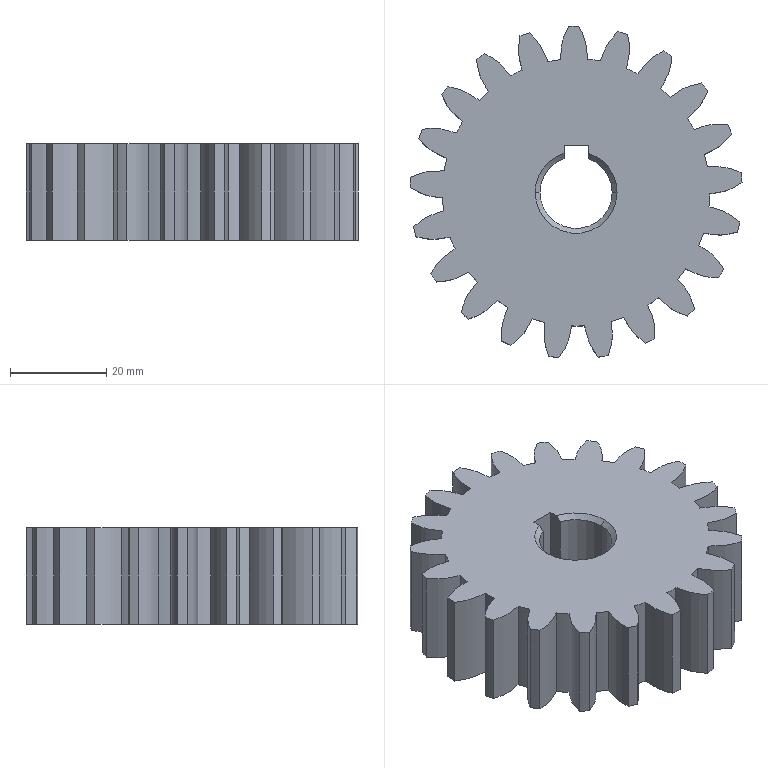Part | SolidWorks | features ICE 2, Chamfer 1, CirPattern 1, Extrusion 1 | 1 solid | 98 faces | box 68.925 x 68.813 x 20 mm | volume 57301 mm3 | cylinder 45 | spline 42 | cone 6 | plane 5 | commonest cylinder face diameters 55.5 x21 69 x21 15 x3